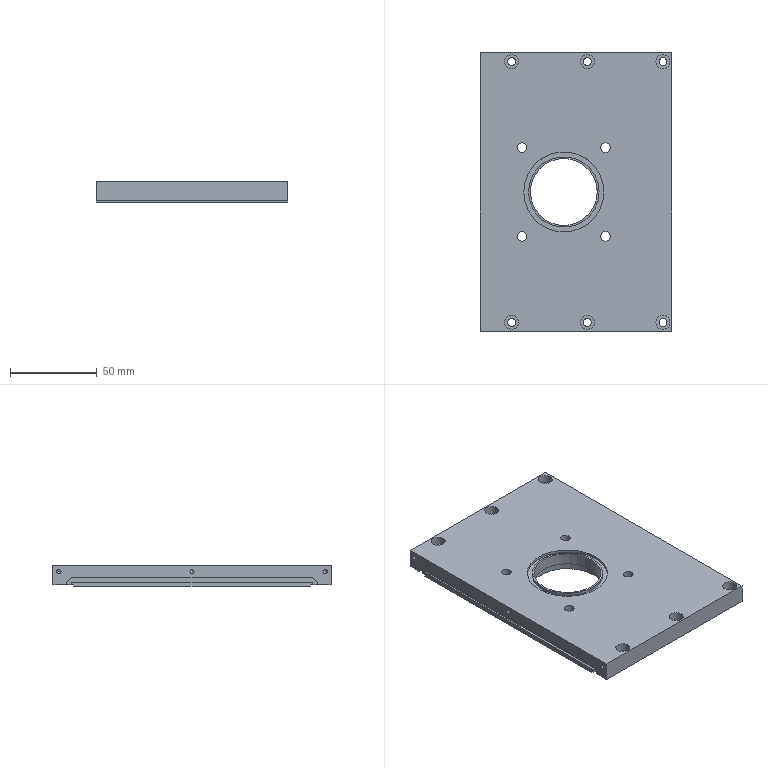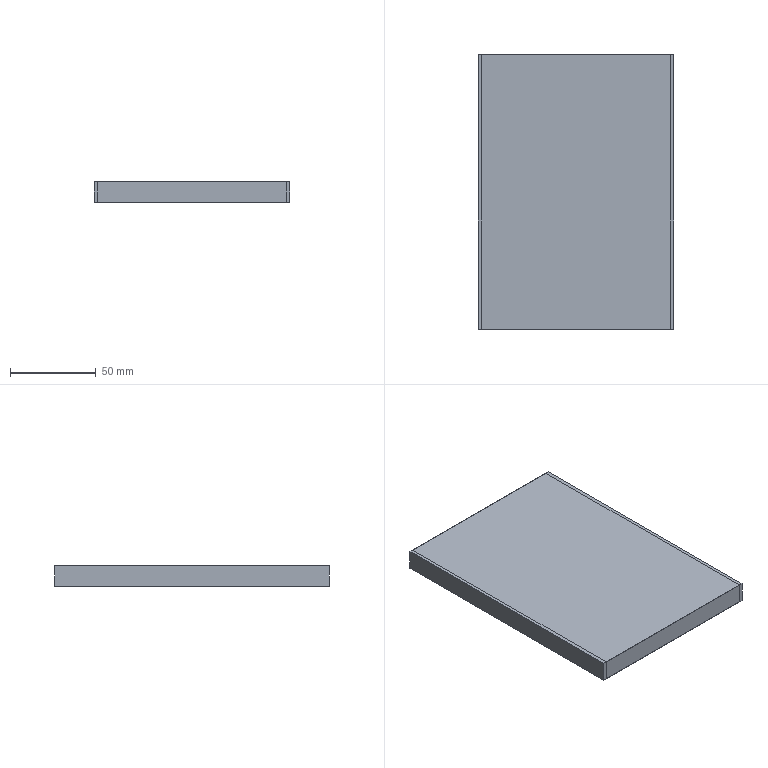CAM job | NX | 3+2 milling, drilling | part box 110 x 160 x 12 mm | stock box 114 x 160 x 12 mm
Tools:
number,name,description,diameter,corner_radius,flute_length,length,flutes
1,D6A45,Milling Tool-5 Parameters,6.0,0.0,50.0,75.0,2
15,D10,Milling Tool-5 Parameters,10.0,0.0,50.0,75.0,2
14,D10JING,Milling Tool-5 Parameters,10.0,0.0,50.0,75.0,2
8,4.5ZT,Drilling Tool,4.5,0.0,35.0,50.0,2
9,5.5ZT,Drilling Tool,5.5,0.0,35.0,50.0,2
11,D4,Milling Tool-5 Parameters,4.0,0.0,50.0,75.0,2
2,D2,Milling Tool-5 Parameters,2.0,0.0,50.0,75.0,2
3,3.3ZT,Drilling Tool,3.2,0.0,35.0,50.0,2
17,D3,Milling Tool-5 Parameters,3.0,0.0,50.0,75.0,2
Operations:
program,operation,operation_type,tool,method,geometry_group,spindle_rpm,surface_speed,feed_per_tooth,feed_cut,feed_plunge,cut_length_mm,path_length_mm,cut_time_min,machine_time_min
1,ZLEVEL_PROFILE_COPY_1_COPY_COPY_1_COPY,ZLevelMilling,D10,METHOD,A,9500.0,298.0,0.1579,3000.0,1000.0,2856.747,4815.263,1.01,1.205
1,FLOOR_WALL,VolumeBased25DMillingOperation,D10,METHOD,A,9500.0,298.0,0.1316,2500.0,1000.0,1002.698,1289.799,0.4049,0.4336
1,HOLE_MILLING,CylinderMilling,D10,METHOD,A,9500.0,298.0,0.1316,2500.0,100.0,1039.242,1103.742,0.4157,0.4221
1,HOLE_MILLING_COPY,CylinderMilling,D10,METHOD,A,9500.0,298.0,0.1316,2500.0,100.0,837.8,914.3,0.3351,0.3428
1,ZLEVEL_PROFILE_COPY_1_COPY_COPY_1,ZLevelMilling,D10JING,METHOD,A,9500.0,298.0,0.0632,1200.0,1000.0,253.953,591.808,0.2129,0.2466
1,ZLEVEL_PROFILE_COPY_1_COPY_COPY_1_COPY_1,ZLevelMilling,D10JING,METHOD,A,9500.0,298.0,0.0632,1200.0,1000.0,111.489,179.489,0.0936,0.1004
1,ZLEVEL_PROFILE_COPY_1_COPY_COPY_1_COPY_1_COPY,ZLevelMilling,D10JING,METHOD,A,9500.0,298.0,0.0632,1200.0,1000.0,97.696,179.696,0.0821,0.0903
1,FLOOR_WALL_1,VolumeBased25DMillingOperation,D10JING,METHOD,A,9500.0,119.0,0.0658,1250.0,100.0,1252.082,1649.655,1.002,1.041
1,DRILLING_COPY_1,Operation,D6A45,METHOD,A,5000.0,94.0,0.035,350.0,0.0,44.0,620.818,0.1257,0.1834
1,DRILLING_COPY_1_COPY_COPY,Operation,4.5ZT,METHOD,A,2000.0,28.0,0.05,200.0,0.0,71.112,543.667,0.3556,0.4028
1,DRILLING_COPY_1_COPY_COPY_COPY,Operation,5.5ZT,METHOD,A,2000.0,28.0,0.05,200.0,0.0,72.609,361.494,0.363,0.3919
1,PLANAR_MILL_COPY_COPY_COPY_COPY_COPY_COPY_1,PlanarMilling,D6A45,METHOD,A,9500.0,179.0,0.0658,1250.0,100.0,712.696,1259.945,0.5702,0.6249
1,PLANAR_MILL_COPY_COPY_COPY_COPY_COPY_COPY_1_COPY,PlanarMilling,D6A45,METHOD,A,9500.0,179.0,0.0658,1250.0,100.0,358.917,1358.713,0.2871,0.3871
2,HOLE_MILLING_1,CylinderMilling,D4,METHOD,B,9500.0,119.0,0.0868,1650.0,100.0,1150.348,1861.348,0.6972,0.7683
2,ZLEVEL_PROFILE,ZLevelMilling,D2,METHOD,B,9500.0,59.0,0.0579,1100.0,100.0,2783.751,2934.645,2.531,2.546
2,PLANAR_MILL_COPY_COPY_COPY_COPY_COPY_COPY_1_COPY_1,PlanarMilling,D6A45,METHOD,B,9500.0,179.0,0.0658,1250.0,100.0,1189.06,2500.935,0.9512,1.082
3,DRILLING_COPY_1_COPY,Operation,D6A45,METHOD,C,5000.0,94.0,0.035,350.0,0.0,16.0,231.429,0.0457,0.0673
3,DRILLING_COPY_1_COPY_COPY_COPY_COPY,Operation,3.3ZT,METHOD,C,2000.0,28.0,0.05,200.0,0.0,41.922,279.982,0.2096,0.2334
3,ZLEVEL_PROFILE_COPY,ZLevelMilling,D3,METHOD,C,6260.0,59.0,0.0879,1100.0,100.0,585.224,801.135,0.532,0.5536
3,PLANAR_MILL_COPY_COPY_COPY_COPY_COPY_COPY_1_COPY_1_COPY,PlanarMilling,D6A45,METHOD,C,9500.0,179.0,0.0658,1250.0,100.0,84.968,508.656,0.068,0.1103
3,刀补17,ZLevelMilling,D3,METHOD,C,9500.0,89.0,0.0526,1000.0,100.0,173.51,390.335,0.1735,0.1952
4,ZLEVEL_PROFILE_COPY_1,ZLevelMilling,D2,METHOD,D,9500.0,59.0,0.0579,1100.0,100.0,2662.357,2723.202,2.42,2.426
4,PLANAR_MILL_COPY_COPY_COPY_COPY_COPY_COPY_1_COPY_1_COPY_COPY,PlanarMilling,D6A45,METHOD,D,9500.0,179.0,0.0658,1250.0,100.0,299.001,357.321,0.2392,0.245